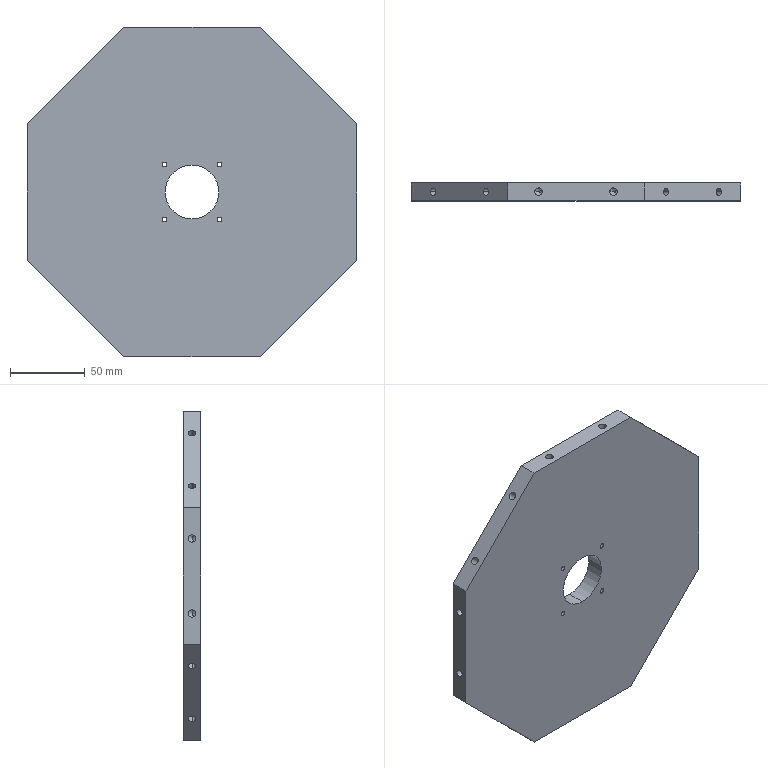Part | SolidWorks | features ICE 3, CirPattern 2, 3DProfileFeature 1, HoleWzd 1, Revolution 1 | 1 solid | 96 faces | box 220 x 12 x 220 mm | volume 463430 mm3 | cylinder 50 | cone 32 | plane 14 | commonest cylinder face diameters 5 x32 3.3 x8 8 x8 36 x2